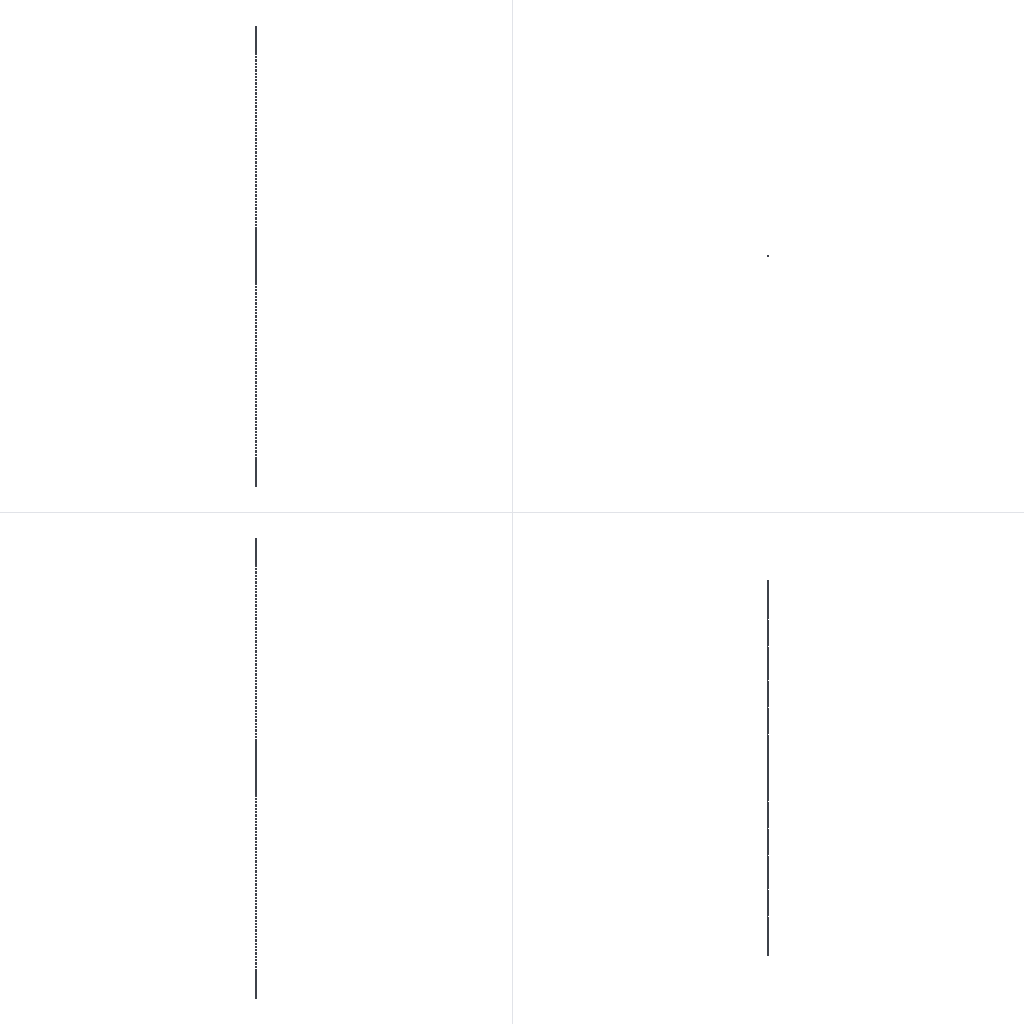Simulation study | abaqus
Set-up summary:
category,name,step,type,value,unit,region
solver,abaqus,,Abaqus/CAE 2024
units,SI m-kg-s (Pa),,inferred,E=1.138e+11 density=4430
analysis,Step-1,,dynamic explicit,nlgeom=True; time_period=0.004
mesh,nodes,,,81764
mesh,elements,,,68289
element_type,C3D8R,,,68289
material,Bar,,E,1.138e+11
material,Bar,,nu,0.345
material,Bar,,density,4430
material,Specimen,,E,2e+08
material,Specimen,,nu,0
material,Specimen,,density,120
section,Bar,,solid section,,,_PickedSet2
section,Specimen,,solid section,,,_PickedSet6
load,Load-1,Step-1,pressure,1.2e+08,,_PickedSurf11
bc,BC-1,Step-1,xsymm,[dofs=XSYMM],,_PickedSet8
bc,BC-2,Step-1,ysymm,[dofs=YSYMM],,_PickedSet9
contact,CP-1-Bar-1-Specimen-1,Step-1,contact pair,interaction=IntProp-1; friction=0; behavior=hard,,CP-1-Bar-1 / _PickedSurf26
contact,CP-2-Bar-2-Specimen-1,Step-1,contact pair,interaction=IntProp-1; friction=0; behavior=hard,,CP-2-Bar-2 / _PickedSurf27
Abaqus input file, long lists of numbers shortened:
*Heading
** Job name: deck Model name: Model-1
** Generated by: Abaqus/CAE 2024
*Preprint, echo=NO, model=NO, history=NO, contact=NO
**
** PARTS
**
*Part, name=Bar
*Node
      1,           0., 0.0066,           7.
      2, -0.0066,           0.,           7.
** (39802 more lines like these left out)
*Element, type=C3D8R
   1,   528,  3908, 14762,  3432,     1,    21,  1766,   272
   2,  3908,  3909, 14763, 14762,    21,    22,  1767,  1766
** (33278 more lines like these left out)
*Nset, nset=_PickedSet2, internal, generate
     1,  39804,      1
*Elset, elset=_PickedSet2, internal, generate
     1,  33280,      1
** Section: Bar
*Solid Section, elset=_PickedSet2, material=Bar
,
*End Part
**
*Part, name=Specimen
*Node
      1, -0.004667, 0.004667, 0.0066
      2, -0.004667, 0.004667,           0.
** (2154 more lines like these left out)
*Element, type=C3D8R
  1,   96,  405, 1005,  345,    1,   15,  201,   50
  2,  405,  406, 1006, 1005,   15,   16,  202,  201
** (1727 more lines like these left out)
*Nset, nset=_PickedSet6, internal, generate
    1,  2156,     1
*Elset, elset=_PickedSet6, internal, generate
    1,  1729,     1
** Section: Specimen
*Solid Section, elset=_PickedSet6, controls=EC-1, material=Specimen
,
*End Part
**
**
** ASSEMBLY
**
*Assembly, name=Assembly
**
*Instance, name=Bar-1, part=Bar
*End Instance
**
*Instance, name=Specimen-1, part=Specimen
-2.07424199344386e-11,           0.,      -0.0066
*End Instance
**
*Instance, name=Bar-2, part=Bar
3.99976596999335e-07,           0.,      -8.007
*End Instance
**
*Nset, nset=Set-6, instance=Specimen-1
   9,  10,  11,  12,  13,  14, 113, 114, 115, 116, 117, 118, 131, 132, 133, 134
 135, 136, 143, 144, 145, 146, 147, 148, 149, 150, 151, 152, 153, 154, 155, 156
** (11 more lines like these left out)
*Elset, elset=Set-6, instance=Specimen-1
  589,  590,  591,  592,  593,  594,  595,  638,  639,  640,  641,  642,  643,  644,  687,  688
  689,  690,  691,  692,  693,  736,  737,  738,  739,  740,  741,  742,  785,  786,  787,  788
** (9 more lines like these left out)
*Nset, nset=Set-7, instance=Specimen-1
   3,   4,   6,   7,  10,  12,  33,  34,  35,  36,  37,  38,  39,  40,  41,  42
  43,  44,  69,  70,  71,  72,  73,  74,  75,  76,  77,  78,  79,  80,  87,  88
** (11 more lines like these left out)
*Elset, elset=Set-7, instance=Specimen-1
   79,   80,   81,   82,   83,   84,   85,   86,   87,   88,   89,   90,   91,  170,  171,  172
  173,  174,  175,  176,  177,  178,  179,  180,  181,  182,  261,  262,  263,  264,  265,  266
** (9 more lines like these left out)
*Nset, nset=_PickedSet8, internal, instance=Bar-1
     1,     4,     7,     8,    10,    11,    13,    14,    15,    16,    17,    20,   154,   155,   156,   157
   158,   159,   160,   161,   162,   163,   164,   165,   166,   167,   168,   169,   170,   171,   172,   173
** (319 more lines like these left out)
*Nset, nset=_PickedSet8, internal, instance=Specimen-1
   9,  10,  11,  12,  13,  14, 113, 114, 115, 116, 117, 118, 131, 132, 133, 134
 135, 136, 143, 144, 145, 146, 147, 148, 149, 150, 151, 152, 153, 154, 155, 156
** (11 more lines like these left out)
*Nset, nset=_PickedSet8, internal, instance=Bar-2
     1,     4,     7,     8,    10,    11,    13,    14,    15,    16,    17,    20,   154,   155,   156,   157
   158,   159,   160,   161,   162,   163,   164,   165,   166,   167,   168,   169,   170,   171,   172,   173
** (319 more lines like these left out)
*Elset, elset=_PickedSet8, internal, instance=Bar-1
     1,     9,    17,    25,    33,    41,    49,    57,    65,    73,    81,    89,    97,   105,   113,   121
   129,   137,   145,   153,   161,   169,   177,   185,   193,   201,   209,   217,   225,   233,   241,   249
** (298 more lines like these left out)
*Elset, elset=_PickedSet8, internal, instance=Specimen-1
  589,  590,  591,  592,  593,  594,  595,  638,  639,  640,  641,  642,  643,  644,  687,  688
  689,  690,  691,  692,  693,  736,  737,  738,  739,  740,  741,  742,  785,  786,  787,  788
** (9 more lines like these left out)
*Elset, elset=_PickedSet8, internal, instance=Bar-2
     1,     9,    17,    25,    33,    41,    49,    57,    65,    73,    81,    89,    97,   105,   113,   121
   129,   137,   145,   153,   161,   169,   177,   185,   193,   201,   209,   217,   225,   233,   241,   249
** (298 more lines like these left out)
*Nset, nset=_PickedSet9, internal, instance=Bar-1
     2,     3,     5,     6,     9,    12,    13,    14,    15,    18,    19,    20,    28,    29,    30,    31
    32,    33,    34,    35,    36,    37,    38,    39,    40,    41,    42,    43,    44,    45,    46,    47
** (319 more lines like these left out)
*Nset, nset=_PickedSet9, internal, instance=Specimen-1
   3,   4,   6,   7,  10,  12,  33,  34,  35,  36,  37,  38,  39,  40,  41,  42
  43,  44,  69,  70,  71,  72,  73,  74,  75,  76,  77,  78,  79,  80,  87,  88
** (11 more lines like these left out)
*Nset, nset=_PickedSet9, internal, instance=Bar-2
     2,     3,     5,     6,     9,    12,    13,    14,    15,    18,    19,    20,    28,    29,    30,    31
    32,    33,    34,    35,    36,    37,    38,    39,    40,    41,    42,    43,    44,    45,    46,    47
** (319 more lines like these left out)
*Elset, elset=_PickedSet9, internal, instance=Bar-1
     8,    16,    24,    32,    40,    48,    56,    64,    72,    80,    88,    96,   104,   112,   120,   128
   136,   144,   152,   160,   168,   176,   184,   192,   200,   208,   216,   224,   232,   240,   248,   256
** (298 more lines like these left out)
*Elset, elset=_PickedSet9, internal, instance=Specimen-1
   79,   80,   81,   82,   83,   84,   85,   86,   87,   88,   89,   90,   91,  170,  171,  172
  173,  174,  175,  176,  177,  178,  179,  180,  181,  182,  261,  262,  263,  264,  265,  266
** (9 more lines like these left out)
*Elset, elset=_PickedSet9, internal, instance=Bar-2
     8,    16,    24,    32,    40,    48,    56,    64,    72,    80,    88,    96,   104,   112,   120,   128
   136,   144,   152,   160,   168,   176,   184,   192,   200,   208,   216,   224,   232,   240,   248,   256
** (298 more lines like these left out)
*Nset, nset=_PickedSet20, internal, instance=Specimen-1, generate
    1,  2156,     1
*Elset, elset=_PickedSet20, internal, instance=Specimen-1, generate
    1,  1729,     1
*Nset, nset=_PickedSet23, internal, instance=Specimen-1, generate
    1,  2156,     1
*Elset, elset=_PickedSet23, internal, instance=Specimen-1, generate
    1,  1729,     1
*Nset, nset=_PickedSet24, internal, instance=Specimen-1, generate
    1,  2156,     1
*Elset, elset=_PickedSet24, internal, instance=Specimen-1, generate
    1,  1729,     1
*Nset, nset=_PickedSet25, internal, instance=Specimen-1, generate
    1,  2156,     1
*Elset, elset=_PickedSet25, internal, instance=Specimen-1, generate
    1,  1729,     1
*Elset, elset=_CP-1-Bar-1_S3, internal, instance=Bar-1
  2881,  2882,  2883,  2884,  2885,  2886,  2887,  2888,  3681,  3682,  3683,  3684,  3685,  3686,  3687,  3688
  4481,  4482,  4483,  4484,  4485,  4486,  4487,  4488, 18881, 18882, 18883, 18884, 19081, 19082, 19083, 19084
** (2 more lines like these left out)
*Elset, elset=_CP-1-Bar-1_S4, internal, instance=Bar-1, generate
 20530,  22080,     50
*Elset, elset=_CP-1-Bar-1_S2, internal, instance=Bar-1, generate
 22081,  22096,      1
*Surface, type=ELEMENT, name=CP-1-Bar-1
_CP-1-Bar-1_S3, S3
_CP-1-Bar-1_S4, S4
_CP-1-Bar-1_S2, S2
*Elset, elset=_CP-1-Specimen-1_S6, internal, instance=Specimen-1
    1,   14,   27,   40,   53,   66,   79,   92,  105,  118,  131,  144,  157,  170,  183,  196
  209,  222,  235,  248,  261,  274,  287,  300,  313,  326,  339,  352,  365,  378,  391,  404
** (4 more lines like these left out)
*Elset, elset=_CP-1-Specimen-1_S1, internal, instance=Specimen-1, generate
 1135,  1183,     1
*Surface, type=ELEMENT, name=CP-1-Specimen-1
_CP-1-Specimen-1_S6, S6
_CP-1-Specimen-1_S1, S1
*Elset, elset=_CP-2-Bar-2_S6, internal, instance=Bar-2, generate
 22881,  25181,    100
*Elset, elset=_CP-2-Bar-2_S2, internal, instance=Bar-2
 25281, 25282, 25283, 25284, 25285, 25286, 25287, 25288, 25289, 25290, 25291, 25292, 25293, 25294, 25295, 25296
 25297, 25298, 25299, 25300, 25301, 25302, 25303, 25304, 25305, 25306, 25307, 25308, 25309, 25310, 25311, 25312
** (3 more lines like these left out)
*Surface, type=ELEMENT, name=CP-2-Bar-2
_CP-2-Bar-2_S6, S6
_CP-2-Bar-2_S2, S2
*Elset, elset=_CP-2-Specimen-1_S4, internal, instance=Specimen-1
   13,   26,   39,   52,   65,   78,   91,  104,  117,  130,  143,  156,  169,  182,  195,  208
  221,  234,  247,  260,  273,  286,  299,  312,  325,  338,  351,  364,  377,  390,  403,  416
** (4 more lines like these left out)
*Elset, elset=_CP-2-Specimen-1_S2, internal, instance=Specimen-1, generate
 547,  595,    1
*Surface, type=ELEMENT, name=CP-2-Specimen-1
_CP-2-Specimen-1_S4, S4
_CP-2-Specimen-1_S2, S2
*Elset, elset=__PickedSurf11_S3, internal, instance=Bar-2
  2881,  2882,  2883,  2884,  2885,  2886,  2887,  2888,  3681,  3682,  3683,  3684,  3685,  3686,  3687,  3688
  4481,  4482,  4483,  4484,  4485,  4486,  4487,  4488, 18881, 18882, 18883, 18884, 19081, 19082, 19083, 19084
** (2 more lines like these left out)
*Elset, elset=__PickedSurf11_S4, internal, instance=Bar-2, generate
 20530,  22080,     50
*Elset, elset=__PickedSurf11_S2, internal, instance=Bar-2, generate
 22081,  22096,      1
*Surface, type=ELEMENT, name=_PickedSurf11, internal
__PickedSurf11_S3, S3
__PickedSurf11_S4, S4
__PickedSurf11_S2, S2
*Elset, elset=__PickedSurf26_S6, internal, instance=Specimen-1
    1,   14,   27,   40,   53,   66,   79,   92,  105,  118,  131,  144,  157,  170,  183,  196
  209,  222,  235,  248,  261,  274,  287,  300,  313,  326,  339,  352,  365,  378,  391,  404
** (9 more lines like these left out)
*Elset, elset=__PickedSurf26_S2, internal, instance=Specimen-1
    1,    2,    3,    4,    5,    6,    7,    8,    9,   10,   11,   12,   13,   14,   15,   16
   17,   18,   19,   20,   21,   22,   23,   24,   25,   26,   27,   28,   29,   30,   31,   32
** (9 more lines like these left out)
*Elset, elset=__PickedSurf26_S5, internal, instance=Specimen-1
   79,   80,   81,   82,   83,   84,   85,   86,   87,   88,   89,   90,   91,  170,  171,  172
  173,  174,  175,  176,  177,  178,  179,  180,  181,  182,  261,  262,  263,  264,  265,  266
** (15 more lines like these left out)
*Elset, elset=__PickedSurf26_S1, internal, instance=Specimen-1, generate
 1135,  1183,     1
*Surface, type=ELEMENT, name=_PickedSurf26, internal
__PickedSurf26_S6, S6
__PickedSurf26_S2, S2
__PickedSurf26_S5, S5
__PickedSurf26_S1, S1
*Elset, elset=__PickedSurf27_S4, internal, instance=Specimen-1
   13,   26,   39,   52,   65,   78,   91,  104,  117,  130,  143,  156,  169,  182,  195,  208
  221,  234,  247,  260,  273,  286,  299,  312,  325,  338,  351,  364,  377,  390,  403,  416
** (4 more lines like these left out)
*Elset, elset=__PickedSurf27_S2, internal, instance=Specimen-1
    1,    2,    3,    4,    5,    6,    7,    8,    9,   10,   11,   12,   13,   14,   15,   16
   17,   18,   19,   20,   21,   22,   23,   24,   25,   26,   27,   28,   29,   30,   31,   32
** (12 more lines like these left out)
*Elset, elset=__PickedSurf27_S5, internal, instance=Specimen-1
   79,   80,   81,   82,   83,   84,   85,   86,   87,   88,   89,   90,   91,  170,  171,  172
  173,  174,  175,  176,  177,  178,  179,  180,  181,  182,  261,  262,  263,  264,  265,  266
** (15 more lines like these left out)
*Elset, elset=__PickedSurf27_S6, internal, instance=Specimen-1, generate
  547,  1177,     7
*Surface, type=ELEMENT, name=_PickedSurf27, internal
__PickedSurf27_S4, S4
__PickedSurf27_S2, S2
__PickedSurf27_S6, S6
__PickedSurf27_S5, S5
*End Assembly
**
** ELEMENT CONTROLS
**
*Section Controls, name=EC-1, hourglass=STIFFNESS
1., 1., 1.
*Amplitude, name=Amp-1
             0.,              0.,        6.43e-06,     0.0004079,       1.286e-05,      0.002377,       1.929e-05,     0.005437
      2.572e-05,     0.009238,       3.215e-05,     0.0137,       3.858e-05,     0.01901,       4.501e-05,     0.0256
      5.144e-05,     0.03402,       5.787e-05,     0.045,        6.43e-05,     0.05939,       7.074e-05,     0.07819
      7.717e-05,     0.1026,        8.36e-05,     0.1339,       9.003e-05,     0.1736,       9.646e-05,     0.2232
     0.0001029,     0.284,      0.0001093,     0.356,      0.0001157,     0.4376,      0.0001222,     0.5253
     0.0001286,     0.6138,      0.000135,     0.6974,      0.0001415,     0.7712,       0.0001479,     0.8321
     0.0001543,     0.8796,      0.0001608,      0.9152,      0.0001672,     0.9413,      0.0001736,     0.9603
     0.0001801,      0.9742,      0.0001865,     0.9844,      0.0001929,     0.9916,      0.0001993,     0.9964
     0.0002058,     0.9991,      0.0002122,              1.,      0.0002186,     0.9991,      0.0002251,     0.9966
      0.0002315,     0.9928,      0.0002379,     0.9885,      0.0002444,     0.9843,      0.0002508,     0.9807
     0.0002572,     0.9779,      0.0002636,      0.9757,      0.0002701,     0.9738,      0.0002765,     0.9719
     0.0002829,     0.9701,      0.0002894,     0.9683,       0.0002958,     0.9669,      0.0003022,     0.9658
     0.0003087,     0.9652,      0.0003151,     0.9649,      0.0003215,     0.9648,      0.0003279,     0.965
     0.0003344,     0.9654,      0.0003408,     0.9658,      0.0003473,     0.9662,      0.0003537,     0.9666
     0.0003601,     0.9671,      0.0003665,     0.9675,      0.000373,     0.968,       0.0003794,     0.9683
     0.0003858,     0.9684,      0.0003923,     0.9685,      0.0003987,     0.9686,      0.0004051,     0.969
     0.0004116,      0.9696,      0.000418,     0.9706,      0.0004244,     0.9716,      0.0004308,      0.9724
     0.0004373,     0.9728,       0.0004437,     0.973,      0.0004501,     0.973,      0.0004566,     0.973
     0.000463,     0.9731,      0.0004694,     0.9731,      0.0004759,     0.973,      0.0004823,     0.9728
     0.0004887,     0.9726,      0.0004951,     0.9723,      0.0005016,     0.9721,      0.000508,     0.972
     0.0005144,     0.9721,      0.0005209,     0.9723,       0.0005273,     0.9726,      0.0005337,     0.9729
     0.0005402,     0.9732,      0.0005466,     0.9733,      0.000553,     0.9734,      0.0005594,     0.9735
     0.0005659,     0.9737,      0.0005723,     0.9739,      0.0005787,     0.9741,      0.0005852,     0.9743
      0.0005916,     0.9744,      0.000598,     0.9745,      0.0006045,     0.9745,       0.0006109,       0.9746
     0.0006173,     0.9747,      0.0006238,     0.9747,      0.0006302,     0.9745,      0.0006366,     0.9741
     0.0006431,     0.9736,      0.0006495,     0.9732,      0.0006559,     0.973,      0.0006623,     0.973
     0.0006688,     0.9732,       0.0006752,     0.9735,      0.0006816,     0.9736,      0.0006881,     0.9737
     0.0006945,     0.9739,      0.0007009,     0.9742,      0.0007074,     0.9745,      0.0007138,     0.9748
     0.0007202,      0.9751,      0.0007266,     0.9754,      0.0007331,     0.9756,      0.0007395,     0.9758
     0.0007459,     0.976,      0.0007524,     0.976,       0.0007588,     0.9759,      0.0007652,     0.9756
     0.0007717,     0.9754,      0.0007781,     0.9754,      0.0007845,     0.9757,      0.000791,     0.9761
     0.0007974,     0.9764,      0.0008038,     0.9765,      0.0008102,     0.9765,      0.0008167,     0.9763
      0.0008231,      0.9763,      0.0008295,      0.9765,      0.000836,     0.9768,      0.0008424,     0.9773
     0.0008488,     0.9777,      0.0008552,     0.9779,      0.0008617,     0.978,      0.0008681,     0.9779
     0.0008745,     0.9778,      0.000881,     0.9775,      0.0008874,     0.9773,      0.0008938,     0.9773
     0.0009003,     0.9774,       0.0009067,     0.9775,      0.0009131,      0.9775,      0.0009196,     0.9772
     0.000926,     0.9766,      0.0009324,     0.976,      0.0009388,     0.9754,      0.0009453,     0.9751
     0.0009517,     0.9749,      0.0009581,     0.9746,      0.0009646,     0.9743,        0.000971,     0.9738
     0.0009774,     0.9735,      0.0009839,     0.9736,      0.0009903,     0.9743,      0.0009967,     0.9754
     0.001003,     0.9768,      0.00101,     0.978,      0.001016,     0.9788,      0.001022,     0.9793
** (10 more lines like these left out)
**
** MATERIALS
**
*Material, name=Bar
*Density
4430.,
*Elastic
 1.138e+11, 0.345
*Material, name=Specimen
*Density
120.,
*Elastic
 2e+08,0.
*Crushable Foam, hardening=ISOTROPIC
 1.05, 0.05
*Crushable Foam Hardening
 1.20026e+06,         0.
 1.20139e+06, 0.002504
 1.20175e+06, 0.007533
 1.20312e+06,  0.01004
 1.20284e+06,  0.01255
 1.20134e+06,  0.01758
 1.20155e+06,  0.02009
 1.20207e+06,   0.0226
 1.20272e+06,  0.02763
 1.20351e+06,  0.03013
 1.20405e+06,  0.03264
 1.20691e+06,  0.03766
 1.20753e+06,  0.04016
 1.20714e+06,  0.04268
 1.20863e+06,  0.0477
 1.20933e+06,  0.0502
 1.20947e+06,   0.05271
 1.21132e+06,  0.05773
 1.21292e+06,  0.06024
 1.21408e+06,  0.06274
 1.21738e+06,  0.06775
 1.21886e+06,   0.07026
 1.21983e+06,  0.07276
 1.22334e+06,  0.07777
 1.22486e+06,   0.08028
 1.22588e+06,  0.08278
   1.228e+06,  0.0878
 1.23025e+06,  0.0903
 1.23247e+06,   0.0928
  1.2354e+06,  0.09781
 1.23698e+06,   0.1003
 1.23898e+06,   0.1028
 1.24433e+06,    0.1078
  1.2479e+06,   0.1103
 1.25016e+06,   0.1128
 1.25127e+06,   0.1178
 1.25335e+06,   0.1203
 1.25548e+06,   0.1228
 1.26029e+06,    0.1278
 1.26233e+06,    0.1303
** (110 more lines like these left out)
*Rate Dependent, type=YIELD RATIO
      1.,     0.
      1., 0.0001
 1.118,  0.001
 1.246,   0.01
 1.414,    0.1
 1.493,     1.
 1.493,   550.
  1.554,  1400.
 1.555,  2200.
**
** INTERACTION PROPERTIES
**
*Surface Interaction, name=IntProp-1
*Friction
0.,
*Surface Behavior, pressure-overclosure=HARD
** ----------------------------------------------------------------
**
** STEP: Step-1
**
*Step, name=Step-1, nlgeom=YES
*Dynamic, Explicit
, 0.004
*Bulk Viscosity
0.06, 1.5
**
** BOUNDARY CONDITIONS
**
** Name: BC-1 Type: Symmetry/Antisymmetry/Encastre
*Boundary
_PickedSet8, XSYMM
** Name: BC-2 Type: Symmetry/Antisymmetry/Encastre
*Boundary
_PickedSet9, YSYMM
**
** LOADS
**
** Name: Load-1   Type: Pressure
*Dsload, amplitude=Amp-1
_PickedSurf11, P, 1.2e+08
**
** INTERACTIONS
**
** Interaction: CP-1-Bar-1-Specimen-1
*Contact Pair, interaction=IntProp-1, mechanical constraint=KINEMATIC, cpset=CP-1-Bar-1-Specimen-1
CP-1-Bar-1, _PickedSurf26
** Interaction: CP-2-Bar-2-Specimen-1
*Contact Pair, interaction=IntProp-1, mechanical constraint=KINEMATIC, cpset=CP-2-Bar-2-Specimen-1
CP-2-Bar-2, _PickedSurf27
**
** OUTPUT REQUESTS
**
*Restart, write, number interval=1, time marks=NO
**
** FIELD OUTPUT: F-Output-1
**
*Output, field, variable=PRESELECT, number interval=50
**
** HISTORY OUTPUT: H-Output-1
**
*Output, history, variable=PRESELECT
*End Step
Results summary:
result,odb.job_status,,,JOB_STATUS_COMPLETED_SUCCESSFULLY,"consistent, unstated (Abaqus has no unit system)"
result,steps[0].procedure,Step-1,,"*DYNAMIC, EXPLICIT","consistent, unstated (Abaqus has no unit system)"
result,steps[0].time_period,Step-1,,0.004,"consistent, unstated (Abaqus has no unit system)"
result,steps[0].n_frames,Step-1,,51,"consistent, unstated (Abaqus has no unit system)"
result,steps[0].last_frame.id,Step-1,,68541,"consistent, unstated (Abaqus has no unit system)"
result,steps[0].last_frame.value,Step-1,,0.004,"consistent, unstated (Abaqus has no unit system)"
result,steps[0].last_frame.description,Step-1,,Increment     68541: Step Time =   4.0000E-03,"consistent, unstated (Abaqus has no unit system)"
result,steps[0].completed,Step-1,,True,"consistent, unstated (Abaqus has no unit system)"
result,steps[0].max_U_magnitude,Step-1,,0.01077,"consistent, unstated (Abaqus has no unit system)"
result,steps[0].max_S_mises,Step-1,,1.37164e+08,"consistent, unstated (Abaqus has no unit system)"
result,steps[0].RF_sum[1],Step-1,,529.389,"consistent, unstated (Abaqus has no unit system)"
result,steps[0].RF_sum[2],Step-1,,387.783,"consistent, unstated (Abaqus has no unit system)"
result,steps[0].RF_sum[3],Step-1,,0,"consistent, unstated (Abaqus has no unit system)"
result,steps[0].diagnostic.n_increments,Step-1,,51,"consistent, unstated (Abaqus has no unit system)"